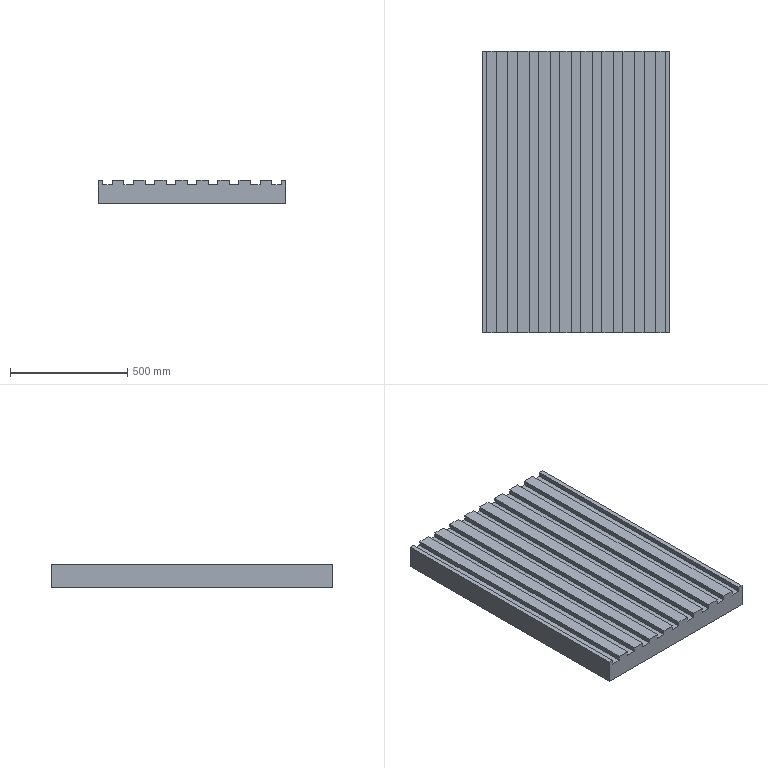Part | SolidWorks | features Extrusion 1, ICE 1, LPattern 1 | 1 solid | 42 faces | box 800 x 1200 x 100 mm | volume 87360000 mm3 | plane 42
STEP:
#1=CARTESIAN_POINT('',(200.,-600.,100.));
#2=VERTEX_POINT('',#1);
#3=CARTESIAN_POINT('',(200.,600.,100.));
#4=VERTEX_POINT('',#3);
#5=CARTESIAN_POINT('',(200.,0.,100.));
#6=DIRECTION('',(0.,1.,0.));
#7=VECTOR('',#6,1000.);
#8=LINE('',#5,#7);
#9=EDGE_CURVE('',#2,#4,#8,.T.);
#10=ORIENTED_EDGE('',*,*,#9,.F.);
#11=CARTESIAN_POINT('',(250.,-600.,100.));
#12=VERTEX_POINT('',#11);
#13=CARTESIAN_POINT('',(-400.,-600.,100.));
#14=DIRECTION('',(1.,0.,0.));
#15=VECTOR('',#14,1000.);
#16=LINE('',#13,#15);
#17=EDGE_CURVE('',#2,#12,#16,.T.);
#18=ORIENTED_EDGE('',*,*,#17,.T.);
#19=CARTESIAN_POINT('',(250.,600.,100.));
#20=VERTEX_POINT('',#19);
#21=CARTESIAN_POINT('',(250.,0.,100.));
#22=DIRECTION('',(0.,-1.,0.));
#23=VECTOR('',#22,1000.);
#24=LINE('',#21,#23);
#25=EDGE_CURVE('',#20,#12,#24,.T.);
#26=ORIENTED_EDGE('',*,*,#25,.F.);
#27=CARTESIAN_POINT('',(-400.,600.,100.));
#28=DIRECTION('',(-1.,0.,0.));
#29=VECTOR('',#28,1000.);
#30=LINE('',#27,#29);
#31=EDGE_CURVE('',#20,#4,#30,.T.);
#32=ORIENTED_EDGE('',*,*,#31,.T.);
#33=EDGE_LOOP('',(#10,#18,#26,#32));
#34=FACE_OUTER_BOUND('',#33,.T.);
#35=CARTESIAN_POINT('',(0.,0.,100.));
#36=DIRECTION('',(0.,0.,1.));
#37=DIRECTION('',(1.,0.,0.));
#38=AXIS2_PLACEMENT_3D('',#35,#36,#37);
#39=PLANE('',#38);
#40=ADVANCED_FACE('',(#34),#39,.T.);
#41=CARTESIAN_POINT('',(290.,-600.,100.));
#42=VERTEX_POINT('',#41);
#43=CARTESIAN_POINT('',(290.,600.,100.));
#44=VERTEX_POINT('',#43);
#45=CARTESIAN_POINT('',(290.,0.,100.));
#46=DIRECTION('',(0.,1.,0.));
#47=VECTOR('',#46,1000.);
#48=LINE('',#45,#47);
#49=EDGE_CURVE('',#42,#44,#48,.T.);
#50=ORIENTED_EDGE('',*,*,#49,.F.);
#51=CARTESIAN_POINT('',(340.,-600.,100.));
#52=VERTEX_POINT('',#51);
#53=CARTESIAN_POINT('',(-400.,-600.,100.));
#54=DIRECTION('',(1.,0.,0.));
#55=VECTOR('',#54,1000.);
#56=LINE('',#53,#55);
#57=EDGE_CURVE('',#42,#52,#56,.T.);
#58=ORIENTED_EDGE('',*,*,#57,.T.);
#59=CARTESIAN_POINT('',(340.,600.,100.));
#60=VERTEX_POINT('',#59);
#61=CARTESIAN_POINT('',(340.,0.,100.));
#62=DIRECTION('',(0.,-1.,0.));
#63=VECTOR('',#62,1000.);
#64=LINE('',#61,#63);
#65=EDGE_CURVE('',#60,#52,#64,.T.);
#66=ORIENTED_EDGE('',*,*,#65,.F.);
#67=CARTESIAN_POINT('',(-400.,600.,100.));
#68=DIRECTION('',(-1.,0.,0.));
#69=VECTOR('',#68,1000.);
#70=LINE('',#67,#69);
#71=EDGE_CURVE('',#60,#44,#70,.T.);
#72=ORIENTED_EDGE('',*,*,#71,.T.);
#73=EDGE_LOOP('',(#50,#58,#66,#72));
#74=FACE_OUTER_BOUND('',#73,.T.);
#75=CARTESIAN_POINT('',(0.,0.,100.));
#76=DIRECTION('',(0.,0.,1.));
#77=DIRECTION('',(1.,0.,0.));
#78=AXIS2_PLACEMENT_3D('',#75,#76,#77);
#79=PLANE('',#78);
#80=ADVANCED_FACE('',(#74),#79,.T.);
#81=CARTESIAN_POINT('',(160.,600.,100.));
#82=VERTEX_POINT('',#81);
#83=CARTESIAN_POINT('',(160.,-600.,100.));
#84=VERTEX_POINT('',#83);
#85=CARTESIAN_POINT('',(160.,0.,100.));
#86=DIRECTION('',(0.,-1.,0.));
#87=VECTOR('',#86,1000.);
#88=LINE('',#85,#87);
#89=EDGE_CURVE('',#82,#84,#88,.T.);
#90=ORIENTED_EDGE('',*,*,#89,.F.);
#91=CARTESIAN_POINT('',(110.,600.,100.));
#92=VERTEX_POINT('',#91);
#93=CARTESIAN_POINT('',(-400.,600.,100.));
#94=DIRECTION('',(-1.,0.,0.));
#95=VECTOR('',#94,1000.);
#96=LINE('',#93,#95);
#97=EDGE_CURVE('',#82,#92,#96,.T.);
#98=ORIENTED_EDGE('',*,*,#97,.T.);
#99=CARTESIAN_POINT('',(110.,-600.,100.));
#100=VERTEX_POINT('',#99);
#101=CARTESIAN_POINT('',(110.,0.,100.));
#102=DIRECTION('',(0.,1.,0.));
#103=VECTOR('',#102,1000.);
#104=LINE('',#101,#103);
#105=EDGE_CURVE('',#100,#92,#104,.T.);
#106=ORIENTED_EDGE('',*,*,#105,.F.);
#107=CARTESIAN_POINT('',(-400.,-600.,100.));
#108=DIRECTION('',(1.,0.,0.));
#109=VECTOR('',#108,1000.);
#110=LINE('',#107,#109);
#111=EDGE_CURVE('',#100,#84,#110,.T.);
#112=ORIENTED_EDGE('',*,*,#111,.T.);
#113=EDGE_LOOP('',(#90,#98,#106,#112));
#114=FACE_OUTER_BOUND('',#113,.T.);
#115=CARTESIAN_POINT('',(0.,0.,100.));
#116=DIRECTION('',(0.,0.,1.));
#117=DIRECTION('',(1.,0.,0.));
#118=AXIS2_PLACEMENT_3D('',#115,#116,#117);
#119=PLANE('',#118);
#120=ADVANCED_FACE('',(#114),#119,.T.);
#121=CARTESIAN_POINT('',(380.,-600.,100.));
#122=VERTEX_POINT('',#121);
#123=CARTESIAN_POINT('',(380.,600.,100.));
#124=VERTEX_POINT('',#123);
#125=CARTESIAN_POINT('',(380.,0.,100.));
#126=DIRECTION('',(0.,1.,0.));
#127=VECTOR('',#126,1000.);
#128=LINE('',#125,#127);
#129=EDGE_CURVE('',#122,#124,#128,.T.);
#130=ORIENTED_EDGE('',*,*,#129,.F.);
#131=CARTESIAN_POINT('',(400.,-600.,100.));
#132=VERTEX_POINT('',#131);
#133=CARTESIAN_POINT('',(-400.,-600.,100.));
#134=DIRECTION('',(1.,0.,0.));
#135=VECTOR('',#134,1000.);
#136=LINE('',#133,#135);
#137=EDGE_CURVE('',#122,#132,#136,.T.);
#138=ORIENTED_EDGE('',*,*,#137,.T.);
#139=CARTESIAN_POINT('',(400.,600.,100.));
#140=VERTEX_POINT('',#139);
#141=CARTESIAN_POINT('',(400.,600.,100.));
#142=DIRECTION('',(0.,1.,0.));
#143=VECTOR('',#142,1000.);
#144=LINE('',#141,#143);
#145=EDGE_CURVE('',#132,#140,#144,.T.);
#146=ORIENTED_EDGE('',*,*,#145,.T.);
#147=CARTESIAN_POINT('',(-400.,600.,100.));
#148=DIRECTION('',(-1.,0.,0.));
#149=VECTOR('',#148,1000.);
#150=LINE('',#147,#149);
#151=EDGE_CURVE('',#140,#124,#150,.T.);
#152=ORIENTED_EDGE('',*,*,#151,.T.);
#153=EDGE_LOOP('',(#130,#138,#146,#152));
#154=FACE_OUTER_BOUND('',#153,.T.);
#155=CARTESIAN_POINT('',(0.,0.,100.));
#156=DIRECTION('',(0.,0.,1.));
#157=DIRECTION('',(1.,0.,0.));
#158=AXIS2_PLACEMENT_3D('',#155,#156,#157);
#159=PLANE('',#158);
#160=ADVANCED_FACE('',(#154),#159,.T.);
#161=CARTESIAN_POINT('',(-340.,-600.,100.));
#162=VERTEX_POINT('',#161);
#163=CARTESIAN_POINT('',(-340.,600.,100.));
#164=VERTEX_POINT('',#163);
#165=CARTESIAN_POINT('',(-340.,0.,100.));
#166=DIRECTION('',(0.,1.,0.));
#167=VECTOR('',#166,1000.);
#168=LINE('',#165,#167);
#169=EDGE_CURVE('',#162,#164,#168,.T.);
#170=ORIENTED_EDGE('',*,*,#169,.F.);
#171=CARTESIAN_POINT('',(-290.,-600.,100.));
#172=VERTEX_POINT('',#171);
#173=CARTESIAN_POINT('',(-400.,-600.,100.));
#174=DIRECTION('',(1.,0.,0.));
#175=VECTOR('',#174,1000.);
#176=LINE('',#173,#175);
#177=EDGE_CURVE('',#162,#172,#176,.T.);
#178=ORIENTED_EDGE('',*,*,#177,.T.);
#179=CARTESIAN_POINT('',(-290.,600.,100.));
#180=VERTEX_POINT('',#179);
#181=CARTESIAN_POINT('',(-290.,0.,100.));
#182=DIRECTION('',(0.,-1.,0.));
#183=VECTOR('',#182,1000.);
#184=LINE('',#181,#183);
#185=EDGE_CURVE('',#180,#172,#184,.T.);
#186=ORIENTED_EDGE('',*,*,#185,.F.);
#187=CARTESIAN_POINT('',(-400.,600.,100.));
#188=DIRECTION('',(-1.,0.,0.));
#189=VECTOR('',#188,1000.);
#190=LINE('',#187,#189);
#191=EDGE_CURVE('',#180,#164,#190,.T.);
#192=ORIENTED_EDGE('',*,*,#191,.T.);
#193=EDGE_LOOP('',(#170,#178,#186,#192));
#194=FACE_OUTER_BOUND('',#193,.T.);
#195=CARTESIAN_POINT('',(0.,0.,100.));
#196=DIRECTION('',(0.,0.,1.));
#197=DIRECTION('',(1.,0.,0.));
#198=AXIS2_PLACEMENT_3D('',#195,#196,#197);
#199=PLANE('',#198);
#200=ADVANCED_FACE('',(#194),#199,.T.);
#201=CARTESIAN_POINT('',(-250.,-600.,100.));
#202=VERTEX_POINT('',#201);
#203=CARTESIAN_POINT('',(-250.,600.,100.));
#204=VERTEX_POINT('',#203);
#205=CARTESIAN_POINT('',(-250.,0.,100.));
#206=DIRECTION('',(0.,1.,0.));
#207=VECTOR('',#206,1000.);
#208=LINE('',#205,#207);
#209=EDGE_CURVE('',#202,#204,#208,.T.);
#210=ORIENTED_EDGE('',*,*,#209,.F.);
#211=CARTESIAN_POINT('',(-200.,-600.,100.));
#212=VERTEX_POINT('',#211);
#213=CARTESIAN_POINT('',(-400.,-600.,100.));
#214=DIRECTION('',(1.,0.,0.));
#215=VECTOR('',#214,1000.);
#216=LINE('',#213,#215);
#217=EDGE_CURVE('',#202,#212,#216,.T.);
#218=ORIENTED_EDGE('',*,*,#217,.T.);
#219=CARTESIAN_POINT('',(-200.,600.,100.));
#220=VERTEX_POINT('',#219);
#221=CARTESIAN_POINT('',(-200.,0.,100.));
#222=DIRECTION('',(0.,-1.,0.));
#223=VECTOR('',#222,1000.);
#224=LINE('',#221,#223);
#225=EDGE_CURVE('',#220,#212,#224,.T.);
#226=ORIENTED_EDGE('',*,*,#225,.F.);
#227=CARTESIAN_POINT('',(-400.,600.,100.));
#228=DIRECTION('',(-1.,0.,0.));
#229=VECTOR('',#228,1000.);
#230=LINE('',#227,#229);
#231=EDGE_CURVE('',#220,#204,#230,.T.);
#232=ORIENTED_EDGE('',*,*,#231,.T.);
#233=EDGE_LOOP('',(#210,#218,#226,#232));
#234=FACE_OUTER_BOUND('',#233,.T.);
#235=CARTESIAN_POINT('',(0.,0.,100.));
#236=DIRECTION('',(0.,0.,1.));
#237=DIRECTION('',(1.,0.,0.));
#238=AXIS2_PLACEMENT_3D('',#235,#236,#237);
#239=PLANE('',#238);
#240=ADVANCED_FACE('',(#234),#239,.T.);
#241=CARTESIAN_POINT('',(-160.,-600.,100.));
#242=VERTEX_POINT('',#241);
#243=CARTESIAN_POINT('',(-160.,600.,100.));
#244=VERTEX_POINT('',#243);
#245=CARTESIAN_POINT('',(-160.,0.,100.));
#246=DIRECTION('',(0.,1.,0.));
#247=VECTOR('',#246,1000.);
#248=LINE('',#245,#247);
#249=EDGE_CURVE('',#242,#244,#248,.T.);
#250=ORIENTED_EDGE('',*,*,#249,.F.);
#251=CARTESIAN_POINT('',(-110.,-600.,100.));
#252=VERTEX_POINT('',#251);
#253=CARTESIAN_POINT('',(-400.,-600.,100.));
#254=DIRECTION('',(1.,0.,0.));
#255=VECTOR('',#254,1000.);
#256=LINE('',#253,#255);
#257=EDGE_CURVE('',#242,#252,#256,.T.);
#258=ORIENTED_EDGE('',*,*,#257,.T.);
#259=CARTESIAN_POINT('',(-110.,600.,100.));
#260=VERTEX_POINT('',#259);
#261=CARTESIAN_POINT('',(-110.,0.,100.));
#262=DIRECTION('',(0.,-1.,0.));
#263=VECTOR('',#262,1000.);
#264=LINE('',#261,#263);
#265=EDGE_CURVE('',#260,#252,#264,.T.);
#266=ORIENTED_EDGE('',*,*,#265,.F.);
#267=CARTESIAN_POINT('',(-400.,600.,100.));
#268=DIRECTION('',(-1.,0.,0.));
#269=VECTOR('',#268,1000.);
#270=LINE('',#267,#269);
#271=EDGE_CURVE('',#260,#244,#270,.T.);
#272=ORIENTED_EDGE('',*,*,#271,.T.);
#273=EDGE_LOOP('',(#250,#258,#266,#272));
#274=FACE_OUTER_BOUND('',#273,.T.);
#275=CARTESIAN_POINT('',(0.,0.,100.));
#276=DIRECTION('',(0.,0.,1.));
#277=DIRECTION('',(1.,0.,0.));
#278=AXIS2_PLACEMENT_3D('',#275,#276,#277);
#279=PLANE('',#278);
#280=ADVANCED_FACE('',(#274),#279,.T.);
#281=CARTESIAN_POINT('',(-70.,-600.,100.));
#282=VERTEX_POINT('',#281);
#283=CARTESIAN_POINT('',(-70.,600.,100.));
#284=VERTEX_POINT('',#283);
#285=CARTESIAN_POINT('',(-70.,0.,100.));
#286=DIRECTION('',(0.,1.,0.));
#287=VECTOR('',#286,1000.);
#288=LINE('',#285,#287);
#289=EDGE_CURVE('',#282,#284,#288,.T.);
#290=ORIENTED_EDGE('',*,*,#289,.F.);
#291=CARTESIAN_POINT('',(-20.,-600.,100.));
#292=VERTEX_POINT('',#291);
#293=CARTESIAN_POINT('',(-400.,-600.,100.));
#294=DIRECTION('',(1.,0.,0.));
#295=VECTOR('',#294,1000.);
#296=LINE('',#293,#295);
#297=EDGE_CURVE('',#282,#292,#296,.T.);
#298=ORIENTED_EDGE('',*,*,#297,.T.);
#299=CARTESIAN_POINT('',(-20.,600.,100.));
#300=VERTEX_POINT('',#299);
#301=CARTESIAN_POINT('',(-20.,0.,100.));
#302=DIRECTION('',(0.,-1.,0.));
#303=VECTOR('',#302,1000.);
#304=LINE('',#301,#303);
#305=EDGE_CURVE('',#300,#292,#304,.T.);
#306=ORIENTED_EDGE('',*,*,#305,.F.);
#307=CARTESIAN_POINT('',(-400.,600.,100.));
#308=DIRECTION('',(-1.,0.,0.));
#309=VECTOR('',#308,1000.);
#310=LINE('',#307,#309);
#311=EDGE_CURVE('',#300,#284,#310,.T.);
#312=ORIENTED_EDGE('',*,*,#311,.T.);
#313=EDGE_LOOP('',(#290,#298,#306,#312));
#314=FACE_OUTER_BOUND('',#313,.T.);
#315=CARTESIAN_POINT('',(0.,0.,100.));
#316=DIRECTION('',(0.,0.,1.));
#317=DIRECTION('',(1.,0.,0.));
#318=AXIS2_PLACEMENT_3D('',#315,#316,#317);
#319=PLANE('',#318);
#320=ADVANCED_FACE('',(#314),#319,.T.);
#321=CARTESIAN_POINT('',(70.,600.,100.));
#322=VERTEX_POINT('',#321);
#323=CARTESIAN_POINT('',(70.,-600.,100.));
#324=VERTEX_POINT('',#323);
#325=CARTESIAN_POINT('',(70.,0.,100.));
#326=DIRECTION('',(0.,-1.,0.));
#327=VECTOR('',#326,1000.);
#328=LINE('',#325,#327);
#329=EDGE_CURVE('',#322,#324,#328,.T.);
#330=ORIENTED_EDGE('',*,*,#329,.F.);
#331=CARTESIAN_POINT('',(20.,600.,100.));
#332=VERTEX_POINT('',#331);
#333=CARTESIAN_POINT('',(-400.,600.,100.));
#334=DIRECTION('',(-1.,0.,0.));
#335=VECTOR('',#334,1000.);
#336=LINE('',#333,#335);
#337=EDGE_CURVE('',#322,#332,#336,.T.);
#338=ORIENTED_EDGE('',*,*,#337,.T.);
#339=CARTESIAN_POINT('',(20.,-600.,100.));
#340=VERTEX_POINT('',#339);
#341=CARTESIAN_POINT('',(20.,0.,100.));
#342=DIRECTION('',(0.,1.,0.));
#343=VECTOR('',#342,1000.);
#344=LINE('',#341,#343);
#345=EDGE_CURVE('',#340,#332,#344,.T.);
#346=ORIENTED_EDGE('',*,*,#345,.F.);
#347=CARTESIAN_POINT('',(-400.,-600.,100.));
#348=DIRECTION('',(1.,0.,0.));
#349=VECTOR('',#348,1000.);
#350=LINE('',#347,#349);
#351=EDGE_CURVE('',#340,#324,#350,.T.);
#352=ORIENTED_EDGE('',*,*,#351,.T.);
#353=EDGE_LOOP('',(#330,#338,#346,#352));
#354=FACE_OUTER_BOUND('',#353,.T.);
#355=CARTESIAN_POINT('',(0.,0.,100.));
#356=DIRECTION('',(0.,0.,1.));
#357=DIRECTION('',(1.,0.,0.));
#358=AXIS2_PLACEMENT_3D('',#355,#356,#357);
#359=PLANE('',#358);
#360=ADVANCED_FACE('',(#354),#359,.T.);
#361=CARTESIAN_POINT('',(400.,-600.,0.));
#362=VERTEX_POINT('',#361);
#363=CARTESIAN_POINT('',(400.,600.,0.));
#364=VERTEX_POINT('',#363);
#365=CARTESIAN_POINT('',(400.,600.,0.));
#366=DIRECTION('',(0.,1.,0.));
#367=VECTOR('',#366,1000.);
#368=LINE('',#365,#367);
#369=EDGE_CURVE('',#362,#364,#368,.T.);
#370=ORIENTED_EDGE('',*,*,#369,.T.);
#371=CARTESIAN_POINT('',(400.,600.,100.));
#372=DIRECTION('',(0.,0.,-1.));
#373=VECTOR('',#372,1000.);
#374=LINE('',#371,#373);
#375=EDGE_CURVE('',#140,#364,#374,.T.);
#376=ORIENTED_EDGE('',*,*,#375,.F.);
#377=ORIENTED_EDGE('',*,*,#145,.F.);
#378=CARTESIAN_POINT('',(400.,-600.,100.));
#379=DIRECTION('',(0.,0.,-1.));
#380=VECTOR('',#379,1000.);
#381=LINE('',#378,#380);
#382=EDGE_CURVE('',#132,#362,#381,.T.);
#383=ORIENTED_EDGE('',*,*,#382,.T.);
#384=EDGE_LOOP('',(#370,#376,#377,#383));
#385=FACE_OUTER_BOUND('',#384,.T.);
#386=CARTESIAN_POINT('',(400.,600.,100.));
#387=DIRECTION('',(-1.,0.,0.));
#388=DIRECTION('',(0.,-1.,0.));
#389=AXIS2_PLACEMENT_3D('',#386,#387,#388);
#390=PLANE('',#389);
#391=ADVANCED_FACE('',(#385),#390,.F.);
#392=CARTESIAN_POINT('',(160.,600.,80.));
#393=VERTEX_POINT('',#392);
#394=CARTESIAN_POINT('',(200.,600.,80.));
#395=VERTEX_POINT('',#394);
#396=CARTESIAN_POINT('',(160.,600.,80.));
#397=DIRECTION('',(1.,0.,0.));
#398=VECTOR('',#397,1000.);
#399=LINE('',#396,#398);
#400=EDGE_CURVE('',#393,#395,#399,.T.);
#401=ORIENTED_EDGE('',*,*,#400,.T.);
#402=CARTESIAN_POINT('',(200.,600.,120.));
#403=DIRECTION('',(0.,0.,1.));
#404=VECTOR('',#403,1000.);
#405=LINE('',#402,#404);
#406=EDGE_CURVE('',#395,#4,#405,.T.);
#407=ORIENTED_EDGE('',*,*,#406,.T.);
#408=ORIENTED_EDGE('',*,*,#31,.F.);
#409=CARTESIAN_POINT('',(250.,600.,80.));
#410=VERTEX_POINT('',#409);
#411=CARTESIAN_POINT('',(250.,600.,120.));
#412=DIRECTION('',(0.,0.,-1.));
#413=VECTOR('',#412,1000.);
#414=LINE('',#411,#413);
#415=EDGE_CURVE('',#20,#410,#414,.T.);
#416=ORIENTED_EDGE('',*,*,#415,.T.);
#417=CARTESIAN_POINT('',(290.,600.,80.));
#418=VERTEX_POINT('',#417);
#419=CARTESIAN_POINT('',(250.,600.,80.));
#420=DIRECTION('',(1.,0.,0.));
#421=VECTOR('',#420,1000.);
#422=LINE('',#419,#421);
#423=EDGE_CURVE('',#410,#418,#422,.T.);
#424=ORIENTED_EDGE('',*,*,#423,.T.);
#425=CARTESIAN_POINT('',(290.,600.,120.));
#426=DIRECTION('',(0.,0.,1.));
#427=VECTOR('',#426,1000.);
#428=LINE('',#425,#427);
#429=EDGE_CURVE('',#418,#44,#428,.T.);
#430=ORIENTED_EDGE('',*,*,#429,.T.);
#431=ORIENTED_EDGE('',*,*,#71,.F.);
#432=CARTESIAN_POINT('',(340.,600.,80.));
#433=VERTEX_POINT('',#432);
#434=CARTESIAN_POINT('',(340.,600.,120.));
#435=DIRECTION('',(0.,0.,-1.));
#436=VECTOR('',#435,1000.);
#437=LINE('',#434,#436);
#438=EDGE_CURVE('',#60,#433,#437,.T.);
#439=ORIENTED_EDGE('',*,*,#438,.T.);
#440=CARTESIAN_POINT('',(380.,600.,80.));
#441=VERTEX_POINT('',#440);
#442=CARTESIAN_POINT('',(340.,600.,80.));
#443=DIRECTION('',(1.,0.,0.));
#444=VECTOR('',#443,1000.);
#445=LINE('',#442,#444);
#446=EDGE_CURVE('',#433,#441,#445,.T.);
#447=ORIENTED_EDGE('',*,*,#446,.T.);
#448=CARTESIAN_POINT('',(380.,600.,120.));
#449=DIRECTION('',(0.,0.,1.));
#450=VECTOR('',#449,1000.);
#451=LINE('',#448,#450);
#452=EDGE_CURVE('',#441,#124,#451,.T.);
#453=ORIENTED_EDGE('',*,*,#452,.T.);
#454=ORIENTED_EDGE('',*,*,#151,.F.);
#455=ORIENTED_EDGE('',*,*,#375,.T.);
#456=CARTESIAN_POINT('',(-400.,600.,0.));
#457=VERTEX_POINT('',#456);
#458=CARTESIAN_POINT('',(-400.,600.,0.));
#459=DIRECTION('',(-1.,0.,0.));
#460=VECTOR('',#459,1000.);
#461=LINE('',#458,#460);
#462=EDGE_CURVE('',#364,#457,#461,.T.);
#463=ORIENTED_EDGE('',*,*,#462,.T.);
#464=CARTESIAN_POINT('',(-400.,600.,100.));
#465=VERTEX_POINT('',#464);
#466=CARTESIAN_POINT('',(-400.,600.,100.));
#467=DIRECTION('',(0.,0.,-1.));
#468=VECTOR('',#467,1000.);
#469=LINE('',#466,#468);
#470=EDGE_CURVE('',#465,#457,#469,.T.);
#471=ORIENTED_EDGE('',*,*,#470,.F.);
#472=CARTESIAN_POINT('',(-380.,600.,100.));
#473=VERTEX_POINT('',#472);
#474=CARTESIAN_POINT('',(-400.,600.,100.));
#475=DIRECTION('',(-1.,0.,0.));
#476=VECTOR('',#475,1000.);
#477=LINE('',#474,#476);
#478=EDGE_CURVE('',#473,#465,#477,.T.);
#479=ORIENTED_EDGE('',*,*,#478,.F.);
#480=CARTESIAN_POINT('',(-380.,600.,80.));
#481=VERTEX_POINT('',#480);
#482=CARTESIAN_POINT('',(-380.,600.,120.));
#483=DIRECTION('',(0.,0.,-1.));
#484=VECTOR('',#483,1000.);
#485=LINE('',#482,#484);
#486=EDGE_CURVE('',#473,#481,#485,.T.);
#487=ORIENTED_EDGE('',*,*,#486,.T.);
#488=CARTESIAN_POINT('',(-340.,600.,80.));
#489=VERTEX_POINT('',#488);
#490=CARTESIAN_POINT('',(-380.,600.,80.));
#491=DIRECTION('',(1.,0.,0.));
#492=VECTOR('',#491,1000.);
#493=LINE('',#490,#492);
#494=EDGE_CURVE('',#481,#489,#493,.T.);
#495=ORIENTED_EDGE('',*,*,#494,.T.);
#496=CARTESIAN_POINT('',(-340.,600.,120.));
#497=DIRECTION('',(0.,0.,1.));
#498=VECTOR('',#497,1000.);
#499=LINE('',#496,#498);
#500=EDGE_CURVE('',#489,#164,#499,.T.);
#501=ORIENTED_EDGE('',*,*,#500,.T.);
#502=ORIENTED_EDGE('',*,*,#191,.F.);
#503=CARTESIAN_POINT('',(-290.,600.,80.));
#504=VERTEX_POINT('',#503);
#505=CARTESIAN_POINT('',(-290.,600.,120.));
#506=DIRECTION('',(0.,0.,-1.));
#507=VECTOR('',#506,1000.);
#508=LINE('',#505,#507);
#509=EDGE_CURVE('',#180,#504,#508,.T.);
#510=ORIENTED_EDGE('',*,*,#509,.T.);
#511=CARTESIAN_POINT('',(-250.,600.,80.));
#512=VERTEX_POINT('',#511);
#513=CARTESIAN_POINT('',(-290.,600.,80.));
#514=DIRECTION('',(1.,0.,0.));
#515=VECTOR('',#514,1000.);
#516=LINE('',#513,#515);
#517=EDGE_CURVE('',#504,#512,#516,.T.);
#518=ORIENTED_EDGE('',*,*,#517,.T.);
#519=CARTESIAN_POINT('',(-250.,600.,120.));
#520=DIRECTION('',(0.,0.,1.));
#521=VECTOR('',#520,1000.);
#522=LINE('',#519,#521);
#523=EDGE_CURVE('',#512,#204,#522,.T.);
#524=ORIENTED_EDGE('',*,*,#523,.T.);
#525=ORIENTED_EDGE('',*,*,#231,.F.);
#526=CARTESIAN_POINT('',(-200.,600.,80.));
#527=VERTEX_POINT('',#526);
#528=CARTESIAN_POINT('',(-200.,600.,120.));
#529=DIRECTION('',(0.,0.,-1.));
#530=VECTOR('',#529,1000.);
#531=LINE('',#528,#530);
#532=EDGE_CURVE('',#220,#527,#531,.T.);
#533=ORIENTED_EDGE('',*,*,#532,.T.);
#534=CARTESIAN_POINT('',(-160.,600.,80.));
#535=VERTEX_POINT('',#534);
#536=CARTESIAN_POINT('',(-200.,600.,80.));
#537=DIRECTION('',(1.,0.,0.));
#538=VECTOR('',#537,1000.);
#539=LINE('',#536,#538);
#540=EDGE_CURVE('',#527,#535,#539,.T.);
#541=ORIENTED_EDGE('',*,*,#540,.T.);
#542=CARTESIAN_POINT('',(-160.,600.,120.));
#543=DIRECTION('',(0.,0.,1.));
#544=VECTOR('',#543,1000.);
#545=LINE('',#542,#544);
#546=EDGE_CURVE('',#535,#244,#545,.T.);
#547=ORIENTED_EDGE('',*,*,#546,.T.);
#548=ORIENTED_EDGE('',*,*,#271,.F.);
#549=CARTESIAN_POINT('',(-110.,600.,80.));
#550=VERTEX_POINT('',#549);
#551=CARTESIAN_POINT('',(-110.,600.,120.));
#552=DIRECTION('',(0.,0.,-1.));
#553=VECTOR('',#552,1000.);
#554=LINE('',#551,#553);
#555=EDGE_CURVE('',#260,#550,#554,.T.);
#556=ORIENTED_EDGE('',*,*,#555,.T.);
#557=CARTESIAN_POINT('',(-70.,600.,80.));
#558=VERTEX_POINT('',#557);
#559=CARTESIAN_POINT('',(-110.,600.,80.));
#560=DIRECTION('',(1.,0.,0.));
#561=VECTOR('',#560,1000.);
#562=LINE('',#559,#561);
#563=EDGE_CURVE('',#550,#558,#562,.T.);
#564=ORIENTED_EDGE('',*,*,#563,.T.);
#565=CARTESIAN_POINT('',(-70.,600.,120.));
#566=DIRECTION('',(0.,0.,1.));
#567=VECTOR('',#566,1000.);
#568=LINE('',#565,#567);
#569=EDGE_CURVE('',#558,#284,#568,.T.);
#570=ORIENTED_EDGE('',*,*,#569,.T.);
#571=ORIENTED_EDGE('',*,*,#311,.F.);
#572=CARTESIAN_POINT('',(-20.,600.,80.));
#573=VERTEX_POINT('',#572);
#574=CARTESIAN_POINT('',(-20.,600.,120.));
#575=DIRECTION('',(0.,0.,-1.));
#576=VECTOR('',#575,1000.);
#577=LINE('',#574,#576);
#578=EDGE_CURVE('',#300,#573,#577,.T.);
#579=ORIENTED_EDGE('',*,*,#578,.T.);
#580=CARTESIAN_POINT('',(20.,600.,80.));
#581=VERTEX_POINT('',#580);
#582=CARTESIAN_POINT('',(-20.,600.,80.));
#583=DIRECTION('',(1.,0.,0.));
#584=VECTOR('',#583,1000.);
#585=LINE('',#582,#584);
#586=EDGE_CURVE('',#573,#581,#585,.T.);
#587=ORIENTED_EDGE('',*,*,#586,.T.);
#588=CARTESIAN_POINT('',(20.,600.,120.));
#589=DIRECTION('',(0.,0.,1.));
#590=VECTOR('',#589,1000.);
#591=LINE('',#588,#590);
#592=EDGE_CURVE('',#581,#332,#591,.T.);
#593=ORIENTED_EDGE('',*,*,#592,.T.);
#594=ORIENTED_EDGE('',*,*,#337,.F.);
#595=CARTESIAN_POINT('',(70.,600.,80.));
#596=VERTEX_POINT('',#595);
#597=CARTESIAN_POINT('',(70.,600.,120.));
#598=DIRECTION('',(0.,0.,-1.));
#599=VECTOR('',#598,1000.);
#600=LINE('',#597,#599);
#601=EDGE_CURVE('',#322,#596,#600,.T.);
#602=ORIENTED_EDGE('',*,*,#601,.T.);
#603=CARTESIAN_POINT('',(110.,600.,80.));
#604=VERTEX_POINT('',#603);
#605=CARTESIAN_POINT('',(70.,600.,80.));
#606=DIRECTION('',(1.,0.,0.));
#607=VECTOR('',#606,1000.);
#608=LINE('',#605,#607);
#609=EDGE_CURVE('',#596,#604,#608,.T.);
#610=ORIENTED_EDGE('',*,*,#609,.T.);
#611=CARTESIAN_POINT('',(110.,600.,120.));
#612=DIRECTION('',(0.,0.,1.));
#613=VECTOR('',#612,1000.);
#614=LINE('',#611,#613);
#615=EDGE_CURVE('',#604,#92,#614,.T.);
#616=ORIENTED_EDGE('',*,*,#615,.T.);
#617=ORIENTED_EDGE('',*,*,#97,.F.);
#618=CARTESIAN_POINT('',(160.,600.,120.));
#619=DIRECTION('',(0.,0.,-1.));
#620=VECTOR('',#619,1000.);
#621=LINE('',#618,#620);
#622=EDGE_CURVE('',#82,#393,#621,.T.);
#623=ORIENTED_EDGE('',*,*,#622,.T.);
#624=EDGE_LOOP('',(#401,#407,#408,#416,#424,#430,#431,#439,#447,#453,#454,#455,#463,#471,#479,#487,#495,#501,#502,#510,#518,#524,#525,#533,#541,#547,#548,#556,#564,#570,#571,#579,#587,#593,#594,#602,#610,#616,#617,#623));
#625=FACE_OUTER_BOUND('',#624,.T.);
#626=CARTESIAN_POINT('',(-400.,600.,100.));
#627=DIRECTION('',(0.,-1.,0.));
#628=DIRECTION('',(0.,0.,-1.));
#629=AXIS2_PLACEMENT_3D('',#626,#627,#628);
#630=PLANE('',#629);
#631=ADVANCED_FACE('',(#625),#630,.F.);
#632=CARTESIAN_POINT('',(-400.,-600.,0.));
#633=VERTEX_POINT('',#632);
#634=CARTESIAN_POINT('',(-400.,600.,0.));
#635=DIRECTION('',(0.,-1.,0.));
#636=VECTOR('',#635,1000.);
#637=LINE('',#634,#636);
#638=EDGE_CURVE('',#457,#633,#637,.T.);
#639=ORIENTED_EDGE('',*,*,#638,.T.);
#640=CARTESIAN_POINT('',(-400.,-600.,100.));
#641=VERTEX_POINT('',#640);
#642=CARTESIAN_POINT('',(-400.,-600.,100.));
#643=DIRECTION('',(0.,0.,-1.));
#644=VECTOR('',#643,1000.);
#645=LINE('',#642,#644);
#646=EDGE_CURVE('',#641,#633,#645,.T.);
#647=ORIENTED_EDGE('',*,*,#646,.F.);
#648=CARTESIAN_POINT('',(-400.,600.,100.));
#649=DIRECTION('',(0.,-1.,0.));
#650=VECTOR('',#649,1000.);
#651=LINE('',#648,#650);
#652=EDGE_CURVE('',#465,#641,#651,.T.);
#653=ORIENTED_EDGE('',*,*,#652,.F.);
#654=ORIENTED_EDGE('',*,*,#470,.T.);
#655=EDGE_LOOP('',(#639,#647,#653,#654));
#656=FACE_OUTER_BOUND('',#655,.T.);
#657=CARTESIAN_POINT('',(-400.,600.,100.));
#658=DIRECTION('',(1.,0.,0.));
#659=DIRECTION('',(0.,1.,0.));
#660=AXIS2_PLACEMENT_3D('',#657,#658,#659);
#661=PLANE('',#660);
#662=ADVANCED_FACE('',(#656),#661,.F.);
#663=ORIENTED_EDGE('',*,*,#17,.F.);
#664=CARTESIAN_POINT('',(200.,-600.,80.));
#665=VERTEX_POINT('',#664);
#666=CARTESIAN_POINT('',(200.,-600.,120.));
#667=DIRECTION('',(0.,0.,1.));
#668=VECTOR('',#667,1000.);
#669=LINE('',#666,#668);
#670=EDGE_CURVE('',#665,#2,#669,.T.);
#671=ORIENTED_EDGE('',*,*,#670,.F.);
#672=CARTESIAN_POINT('',(160.,-600.,80.));
#673=VERTEX_POINT('',#672);
#674=CARTESIAN_POINT('',(160.,-600.,80.));
#675=DIRECTION('',(1.,0.,0.));
#676=VECTOR('',#675,1000.);
#677=LINE('',#674,#676);
#678=EDGE_CURVE('',#673,#665,#677,.T.);
#679=ORIENTED_EDGE('',*,*,#678,.F.);
#680=CARTESIAN_POINT('',(160.,-600.,100.));
#681=DIRECTION('',(0.,0.,1.));
#682=VECTOR('',#681,1000.);
#683=LINE('',#680,#682);
#684=EDGE_CURVE('',#673,#84,#683,.T.);
#685=ORIENTED_EDGE('',*,*,#684,.T.);
#686=ORIENTED_EDGE('',*,*,#111,.F.);
#687=CARTESIAN_POINT('',(110.,-600.,80.));
#688=VERTEX_POINT('',#687);
#689=CARTESIAN_POINT('',(110.,-600.,120.));
#690=DIRECTION('',(0.,0.,1.));
#691=VECTOR('',#690,1000.);
#692=LINE('',#689,#691);
#693=EDGE_CURVE('',#688,#100,#692,.T.);
#694=ORIENTED_EDGE('',*,*,#693,.F.);
#695=CARTESIAN_POINT('',(70.,-600.,80.));
#696=VERTEX_POINT('',#695);
#697=CARTESIAN_POINT('',(70.,-600.,80.));
#698=DIRECTION('',(1.,0.,0.));
#699=VECTOR('',#698,1000.);
#700=LINE('',#697,#699);
#701=EDGE_CURVE('',#696,#688,#700,.T.);
#702=ORIENTED_EDGE('',*,*,#701,.F.);
#703=CARTESIAN_POINT('',(70.,-600.,100.));
#704=DIRECTION('',(0.,0.,1.));
#705=VECTOR('',#704,1000.);
#706=LINE('',#703,#705);
#707=EDGE_CURVE('',#696,#324,#706,.T.);
#708=ORIENTED_EDGE('',*,*,#707,.T.);
#709=ORIENTED_EDGE('',*,*,#351,.F.);
#710=CARTESIAN_POINT('',(20.,-600.,80.));
#711=VERTEX_POINT('',#710);
#712=CARTESIAN_POINT('',(20.,-600.,120.));
#713=DIRECTION('',(0.,0.,1.));
#714=VECTOR('',#713,1000.);
#715=LINE('',#712,#714);
#716=EDGE_CURVE('',#711,#340,#715,.T.);
#717=ORIENTED_EDGE('',*,*,#716,.F.);
#718=CARTESIAN_POINT('',(-20.,-600.,80.));
#719=VERTEX_POINT('',#718);
#720=CARTESIAN_POINT('',(-20.,-600.,80.));
#721=DIRECTION('',(1.,0.,0.));
#722=VECTOR('',#721,1000.);
#723=LINE('',#720,#722);
#724=EDGE_CURVE('',#719,#711,#723,.T.);
#725=ORIENTED_EDGE('',*,*,#724,.F.);
#726=CARTESIAN_POINT('',(-20.,-600.,120.));
#727=DIRECTION('',(0.,0.,-1.));
#728=VECTOR('',#727,1000.);
#729=LINE('',#726,#728);
#730=EDGE_CURVE('',#292,#719,#729,.T.);
#731=ORIENTED_EDGE('',*,*,#730,.F.);
#732=ORIENTED_EDGE('',*,*,#297,.F.);
#733=CARTESIAN_POINT('',(-70.,-600.,80.));
#734=VERTEX_POINT('',#733);
#735=CARTESIAN_POINT('',(-70.,-600.,120.));
#736=DIRECTION('',(0.,0.,1.));
#737=VECTOR('',#736,1000.);
#738=LINE('',#735,#737);
#739=EDGE_CURVE('',#734,#282,#738,.T.);
#740=ORIENTED_EDGE('',*,*,#739,.F.);
#741=CARTESIAN_POINT('',(-110.,-600.,80.));
#742=VERTEX_POINT('',#741);
#743=CARTESIAN_POINT('',(-110.,-600.,80.));
#744=DIRECTION('',(1.,0.,0.));
#745=VECTOR('',#744,1000.);
#746=LINE('',#743,#745);
#747=EDGE_CURVE('',#742,#734,#746,.T.);
#748=ORIENTED_EDGE('',*,*,#747,.F.);
#749=CARTESIAN_POINT('',(-110.,-600.,120.));
#750=DIRECTION('',(0.,0.,-1.));
#751=VECTOR('',#750,1000.);
#752=LINE('',#749,#751);
#753=EDGE_CURVE('',#252,#742,#752,.T.);
#754=ORIENTED_EDGE('',*,*,#753,.F.);
#755=ORIENTED_EDGE('',*,*,#257,.F.);
#756=CARTESIAN_POINT('',(-160.,-600.,80.));
#757=VERTEX_POINT('',#756);
#758=CARTESIAN_POINT('',(-160.,-600.,120.));
#759=DIRECTION('',(0.,0.,1.));
#760=VECTOR('',#759,1000.);
#761=LINE('',#758,#760);
#762=EDGE_CURVE('',#757,#242,#761,.T.);
#763=ORIENTED_EDGE('',*,*,#762,.F.);
#764=CARTESIAN_POINT('',(-200.,-600.,80.));
#765=VERTEX_POINT('',#764);
#766=CARTESIAN_POINT('',(-200.,-600.,80.));
#767=DIRECTION('',(1.,0.,0.));
#768=VECTOR('',#767,1000.);
#769=LINE('',#766,#768);
#770=EDGE_CURVE('',#765,#757,#769,.T.);
#771=ORIENTED_EDGE('',*,*,#770,.F.);
#772=CARTESIAN_POINT('',(-200.,-600.,120.));
#773=DIRECTION('',(0.,0.,-1.));
#774=VECTOR('',#773,1000.);
#775=LINE('',#772,#774);
#776=EDGE_CURVE('',#212,#765,#775,.T.);
#777=ORIENTED_EDGE('',*,*,#776,.F.);
#778=ORIENTED_EDGE('',*,*,#217,.F.);
#779=CARTESIAN_POINT('',(-250.,-600.,80.));
#780=VERTEX_POINT('',#779);
#781=CARTESIAN_POINT('',(-250.,-600.,120.));
#782=DIRECTION('',(0.,0.,1.));
#783=VECTOR('',#782,1000.);
#784=LINE('',#781,#783);
#785=EDGE_CURVE('',#780,#202,#784,.T.);
#786=ORIENTED_EDGE('',*,*,#785,.F.);
#787=CARTESIAN_POINT('',(-290.,-600.,80.));
#788=VERTEX_POINT('',#787);
#789=CARTESIAN_POINT('',(-290.,-600.,80.));
#790=DIRECTION('',(1.,0.,0.));
#791=VECTOR('',#790,1000.);
#792=LINE('',#789,#791);
#793=EDGE_CURVE('',#788,#780,#792,.T.);
#794=ORIENTED_EDGE('',*,*,#793,.F.);
#795=CARTESIAN_POINT('',(-290.,-600.,120.));
#796=DIRECTION('',(0.,0.,-1.));
#797=VECTOR('',#796,1000.);
#798=LINE('',#795,#797);
#799=EDGE_CURVE('',#172,#788,#798,.T.);
#800=ORIENTED_EDGE('',*,*,#799,.F.);
#801=ORIENTED_EDGE('',*,*,#177,.F.);
#802=CARTESIAN_POINT('',(-340.,-600.,80.));
#803=VERTEX_POINT('',#802);
#804=CARTESIAN_POINT('',(-340.,-600.,120.));
#805=DIRECTION('',(0.,0.,1.));
#806=VECTOR('',#805,1000.);
#807=LINE('',#804,#806);
#808=EDGE_CURVE('',#803,#162,#807,.T.);
#809=ORIENTED_EDGE('',*,*,#808,.F.);
#810=CARTESIAN_POINT('',(-380.,-600.,80.));
#811=VERTEX_POINT('',#810);
#812=CARTESIAN_POINT('',(-380.,-600.,80.));
#813=DIRECTION('',(1.,0.,0.));
#814=VECTOR('',#813,1000.);
#815=LINE('',#812,#814);
#816=EDGE_CURVE('',#811,#803,#815,.T.);
#817=ORIENTED_EDGE('',*,*,#816,.F.);
#818=CARTESIAN_POINT('',(-380.,-600.,100.));
#819=VERTEX_POINT('',#818);
#820=CARTESIAN_POINT('',(-380.,-600.,120.));
#821=DIRECTION('',(0.,0.,-1.));
#822=VECTOR('',#821,1000.);
#823=LINE('',#820,#822);
#824=EDGE_CURVE('',#819,#811,#823,.T.);
#825=ORIENTED_EDGE('',*,*,#824,.F.);
#826=CARTESIAN_POINT('',(-400.,-600.,100.));
#827=DIRECTION('',(1.,0.,0.));
#828=VECTOR('',#827,1000.);
#829=LINE('',#826,#828);
#830=EDGE_CURVE('',#641,#819,#829,.T.);
#831=ORIENTED_EDGE('',*,*,#830,.F.);
#832=ORIENTED_EDGE('',*,*,#646,.T.);
#833=CARTESIAN_POINT('',(-400.,-600.,0.));
#834=DIRECTION('',(1.,0.,0.));
#835=VECTOR('',#834,1000.);
#836=LINE('',#833,#835);
#837=EDGE_CURVE('',#633,#362,#836,.T.);
#838=ORIENTED_EDGE('',*,*,#837,.T.);
#839=ORIENTED_EDGE('',*,*,#382,.F.);
#840=ORIENTED_EDGE('',*,*,#137,.F.);
#841=CARTESIAN_POINT('',(380.,-600.,80.));
#842=VERTEX_POINT('',#841);
#843=CARTESIAN_POINT('',(380.,-600.,120.));
#844=DIRECTION('',(0.,0.,1.));
#845=VECTOR('',#844,1000.);
#846=LINE('',#843,#845);
#847=EDGE_CURVE('',#842,#122,#846,.T.);
#848=ORIENTED_EDGE('',*,*,#847,.F.);
#849=CARTESIAN_POINT('',(340.,-600.,80.));
#850=VERTEX_POINT('',#849);
#851=CARTESIAN_POINT('',(340.,-600.,80.));
#852=DIRECTION('',(1.,0.,0.));
#853=VECTOR('',#852,1000.);
#854=LINE('',#851,#853);
#855=EDGE_CURVE('',#850,#842,#854,.T.);
#856=ORIENTED_EDGE('',*,*,#855,.F.);
#857=CARTESIAN_POINT('',(340.,-600.,100.));
#858=DIRECTION('',(0.,0.,1.));
#859=VECTOR('',#858,1000.);
#860=LINE('',#857,#859);
#861=EDGE_CURVE('',#850,#52,#860,.T.);
#862=ORIENTED_EDGE('',*,*,#861,.T.);
#863=ORIENTED_EDGE('',*,*,#57,.F.);
#864=CARTESIAN_POINT('',(290.,-600.,80.));
#865=VERTEX_POINT('',#864);
#866=CARTESIAN_POINT('',(290.,-600.,120.));
#867=DIRECTION('',(0.,0.,1.));
#868=VECTOR('',#867,1000.);
#869=LINE('',#866,#868);
#870=EDGE_CURVE('',#865,#42,#869,.T.);
#871=ORIENTED_EDGE('',*,*,#870,.F.);
#872=CARTESIAN_POINT('',(250.,-600.,80.));
#873=VERTEX_POINT('',#872);
#874=CARTESIAN_POINT('',(250.,-600.,80.));
#875=DIRECTION('',(1.,0.,0.));
#876=VECTOR('',#875,1000.);
#877=LINE('',#874,#876);
#878=EDGE_CURVE('',#873,#865,#877,.T.);
#879=ORIENTED_EDGE('',*,*,#878,.F.);
#880=CARTESIAN_POINT('',(250.,-600.,100.));
#881=DIRECTION('',(0.,0.,1.));
#882=VECTOR('',#881,1000.);
#883=LINE('',#880,#882);
#884=EDGE_CURVE('',#873,#12,#883,.T.);
#885=ORIENTED_EDGE('',*,*,#884,.T.);
#886=EDGE_LOOP('',(#663,#671,#679,#685,#686,#694,#702,#708,#709,#717,#725,#731,#732,#740,#748,#754,#755,#763,#771,#777,#778,#786,#794,#800,#801,#809,#817,#825,#831,#832,#838,#839,#840,#848,#856,#862,#863,#871,#879,#885));
#887=FACE_OUTER_BOUND('',#886,.T.);
#888=CARTESIAN_POINT('',(-400.,-600.,100.));
#889=DIRECTION('',(0.,1.,0.));
#890=DIRECTION('',(0.,0.,1.));
#891=AXIS2_PLACEMENT_3D('',#888,#889,#890);
#892=PLANE('',#891);
#893=ADVANCED_FACE('',(#887),#892,.F.);
#894=CARTESIAN_POINT('',(-380.,0.,100.));
#895=DIRECTION('',(0.,-1.,0.));
#896=VECTOR('',#895,1000.);
#897=LINE('',#894,#896);
#898=EDGE_CURVE('',#473,#819,#897,.T.);
#899=ORIENTED_EDGE('',*,*,#898,.F.);
#900=ORIENTED_EDGE('',*,*,#478,.T.);
#901=ORIENTED_EDGE('',*,*,#652,.T.);
#902=ORIENTED_EDGE('',*,*,#830,.T.);
#903=EDGE_LOOP('',(#899,#900,#901,#902));
#904=FACE_OUTER_BOUND('',#903,.T.);
#905=CARTESIAN_POINT('',(0.,0.,100.));
#906=DIRECTION('',(0.,0.,1.));
#907=DIRECTION('',(1.,0.,0.));
#908=AXIS2_PLACEMENT_3D('',#905,#906,#907);
#909=PLANE('',#908);
#910=ADVANCED_FACE('',(#904),#909,.T.);
#911=ORIENTED_EDGE('',*,*,#369,.F.);
#912=ORIENTED_EDGE('',*,*,#837,.F.);
#913=ORIENTED_EDGE('',*,*,#638,.F.);
#914=ORIENTED_EDGE('',*,*,#462,.F.);
#915=EDGE_LOOP('',(#911,#912,#913,#914));
#916=FACE_OUTER_BOUND('',#915,.T.);
#917=CARTESIAN_POINT('',(0.,0.,0.));
#918=DIRECTION('',(0.,0.,1.));
#919=DIRECTION('',(1.,0.,0.));
#920=AXIS2_PLACEMENT_3D('',#917,#918,#919);
#921=PLANE('',#920);
#922=ADVANCED_FACE('',(#916),#921,.F.);
#923=ORIENTED_EDGE('',*,*,#345,.T.);
#924=ORIENTED_EDGE('',*,*,#592,.F.);
#925=CARTESIAN_POINT('',(20.,600.,80.));
#926=DIRECTION('',(0.,-1.,0.));
#927=VECTOR('',#926,1000.);
#928=LINE('',#925,#927);
#929=EDGE_CURVE('',#581,#711,#928,.T.);
#930=ORIENTED_EDGE('',*,*,#929,.T.);
#931=ORIENTED_EDGE('',*,*,#716,.T.);
#932=EDGE_LOOP('',(#923,#924,#930,#931));
#933=FACE_OUTER_BOUND('',#932,.T.);
#934=CARTESIAN_POINT('',(20.,600.,120.));
#935=DIRECTION('',(1.,0.,0.));
#936=DIRECTION('',(0.,0.,-1.));
#937=AXIS2_PLACEMENT_3D('',#934,#935,#936);
#938=PLANE('',#937);
#939=ADVANCED_FACE('',(#933),#938,.F.);
#940=ORIENTED_EDGE('',*,*,#724,.T.);
#941=ORIENTED_EDGE('',*,*,#929,.F.);
#942=ORIENTED_EDGE('',*,*,#586,.F.);
#943=CARTESIAN_POINT('',(-20.,600.,80.));
#944=DIRECTION('',(0.,-1.,0.));
#945=VECTOR('',#944,1000.);
#946=LINE('',#943,#945);
#947=EDGE_CURVE('',#573,#719,#946,.T.);
#948=ORIENTED_EDGE('',*,*,#947,.T.);
#949=EDGE_LOOP('',(#940,#941,#942,#948));
#950=FACE_OUTER_BOUND('',#949,.T.);
#951=CARTESIAN_POINT('',(-20.,600.,80.));
#952=DIRECTION('',(0.,0.,-1.));
#953=DIRECTION('',(-1.,0.,0.));
#954=AXIS2_PLACEMENT_3D('',#951,#952,#953);
#955=PLANE('',#954);
#956=ADVANCED_FACE('',(#950),#955,.F.);
#957=ORIENTED_EDGE('',*,*,#305,.T.);
#958=ORIENTED_EDGE('',*,*,#730,.T.);
#959=ORIENTED_EDGE('',*,*,#947,.F.);
#960=ORIENTED_EDGE('',*,*,#578,.F.);
#961=EDGE_LOOP('',(#957,#958,#959,#960));
#962=FACE_OUTER_BOUND('',#961,.T.);
#963=CARTESIAN_POINT('',(-20.,600.,120.));
#964=DIRECTION('',(-1.,0.,0.));
#965=DIRECTION('',(0.,0.,1.));
#966=AXIS2_PLACEMENT_3D('',#963,#964,#965);
#967=PLANE('',#966);
#968=ADVANCED_FACE('',(#962),#967,.F.);
#969=ORIENTED_EDGE('',*,*,#289,.T.);
#970=ORIENTED_EDGE('',*,*,#569,.F.);
#971=CARTESIAN_POINT('',(-70.,600.,80.));
#972=DIRECTION('',(0.,-1.,0.));
#973=VECTOR('',#972,1000.);
#974=LINE('',#971,#973);
#975=EDGE_CURVE('',#558,#734,#974,.T.);
#976=ORIENTED_EDGE('',*,*,#975,.T.);
#977=ORIENTED_EDGE('',*,*,#739,.T.);
#978=EDGE_LOOP('',(#969,#970,#976,#977));
#979=FACE_OUTER_BOUND('',#978,.T.);
#980=CARTESIAN_POINT('',(-70.,600.,120.));
#981=DIRECTION('',(1.,0.,0.));
#982=DIRECTION('',(0.,0.,-1.));
#983=AXIS2_PLACEMENT_3D('',#980,#981,#982);
#984=PLANE('',#983);
#985=ADVANCED_FACE('',(#979),#984,.F.);
#986=ORIENTED_EDGE('',*,*,#747,.T.);
#987=ORIENTED_EDGE('',*,*,#975,.F.);
#988=ORIENTED_EDGE('',*,*,#563,.F.);
#989=CARTESIAN_POINT('',(-110.,600.,80.));
#990=DIRECTION('',(0.,-1.,0.));
#991=VECTOR('',#990,1000.);
#992=LINE('',#989,#991);
#993=EDGE_CURVE('',#550,#742,#992,.T.);
#994=ORIENTED_EDGE('',*,*,#993,.T.);
#995=EDGE_LOOP('',(#986,#987,#988,#994));
#996=FACE_OUTER_BOUND('',#995,.T.);
#997=CARTESIAN_POINT('',(-110.,600.,80.));
#998=DIRECTION('',(0.,0.,-1.));
#999=DIRECTION('',(-1.,0.,0.));
#1000=AXIS2_PLACEMENT_3D('',#997,#998,#999);
#1001=PLANE('',#1000);
#1002=ADVANCED_FACE('',(#996),#1001,.F.);
#1003=ORIENTED_EDGE('',*,*,#265,.T.);
#1004=ORIENTED_EDGE('',*,*,#753,.T.);
#1005=ORIENTED_EDGE('',*,*,#993,.F.);
#1006=ORIENTED_EDGE('',*,*,#555,.F.);
#1007=EDGE_LOOP('',(#1003,#1004,#1005,#1006));
#1008=FACE_OUTER_BOUND('',#1007,.T.);
#1009=CARTESIAN_POINT('',(-110.,600.,120.));
#1010=DIRECTION('',(-1.,0.,0.));
#1011=DIRECTION('',(0.,0.,1.));
#1012=AXIS2_PLACEMENT_3D('',#1009,#1010,#1011);
#1013=PLANE('',#1012);
#1014=ADVANCED_FACE('',(#1008),#1013,.F.);
#1015=ORIENTED_EDGE('',*,*,#249,.T.);
#1016=ORIENTED_EDGE('',*,*,#546,.F.);
#1017=CARTESIAN_POINT('',(-160.,600.,80.));
#1018=DIRECTION('',(0.,-1.,0.));
#1019=VECTOR('',#1018,1000.);
#1020=LINE('',#1017,#1019);
#1021=EDGE_CURVE('',#535,#757,#1020,.T.);
#1022=ORIENTED_EDGE('',*,*,#1021,.T.);
#1023=ORIENTED_EDGE('',*,*,#762,.T.);
#1024=EDGE_LOOP('',(#1015,#1016,#1022,#1023));
#1025=FACE_OUTER_BOUND('',#1024,.T.);
#1026=CARTESIAN_POINT('',(-160.,600.,120.));
#1027=DIRECTION('',(1.,0.,0.));
#1028=DIRECTION('',(0.,0.,-1.));
#1029=AXIS2_PLACEMENT_3D('',#1026,#1027,#1028);
#1030=PLANE('',#1029);
#1031=ADVANCED_FACE('',(#1025),#1030,.F.);
#1032=ORIENTED_EDGE('',*,*,#770,.T.);
#1033=ORIENTED_EDGE('',*,*,#1021,.F.);
#1034=ORIENTED_EDGE('',*,*,#540,.F.);
#1035=CARTESIAN_POINT('',(-200.,600.,80.));
#1036=DIRECTION('',(0.,-1.,0.));
#1037=VECTOR('',#1036,1000.);
#1038=LINE('',#1035,#1037);
#1039=EDGE_CURVE('',#527,#765,#1038,.T.);
#1040=ORIENTED_EDGE('',*,*,#1039,.T.);
#1041=EDGE_LOOP('',(#1032,#1033,#1034,#1040));
#1042=FACE_OUTER_BOUND('',#1041,.T.);
#1043=CARTESIAN_POINT('',(-200.,600.,80.));
#1044=DIRECTION('',(0.,0.,-1.));
#1045=DIRECTION('',(-1.,0.,0.));
#1046=AXIS2_PLACEMENT_3D('',#1043,#1044,#1045);
#1047=PLANE('',#1046);
#1048=ADVANCED_FACE('',(#1042),#1047,.F.);
#1049=ORIENTED_EDGE('',*,*,#225,.T.);
#1050=ORIENTED_EDGE('',*,*,#776,.T.);
#1051=ORIENTED_EDGE('',*,*,#1039,.F.);
#1052=ORIENTED_EDGE('',*,*,#532,.F.);
#1053=EDGE_LOOP('',(#1049,#1050,#1051,#1052));
#1054=FACE_OUTER_BOUND('',#1053,.T.);
#1055=CARTESIAN_POINT('',(-200.,600.,120.));
#1056=DIRECTION('',(-1.,0.,0.));
#1057=DIRECTION('',(0.,0.,1.));
#1058=AXIS2_PLACEMENT_3D('',#1055,#1056,#1057);
#1059=PLANE('',#1058);
#1060=ADVANCED_FACE('',(#1054),#1059,.F.);
#1061=ORIENTED_EDGE('',*,*,#209,.T.);
#1062=ORIENTED_EDGE('',*,*,#523,.F.);
#1063=CARTESIAN_POINT('',(-250.,600.,80.));
#1064=DIRECTION('',(0.,-1.,0.));
#1065=VECTOR('',#1064,1000.);
#1066=LINE('',#1063,#1065);
#1067=EDGE_CURVE('',#512,#780,#1066,.T.);
#1068=ORIENTED_EDGE('',*,*,#1067,.T.);
#1069=ORIENTED_EDGE('',*,*,#785,.T.);
#1070=EDGE_LOOP('',(#1061,#1062,#1068,#1069));
#1071=FACE_OUTER_BOUND('',#1070,.T.);
#1072=CARTESIAN_POINT('',(-250.,600.,120.));
#1073=DIRECTION('',(1.,0.,0.));
#1074=DIRECTION('',(0.,0.,-1.));
#1075=AXIS2_PLACEMENT_3D('',#1072,#1073,#1074);
#1076=PLANE('',#1075);
#1077=ADVANCED_FACE('',(#1071),#1076,.F.);
#1078=ORIENTED_EDGE('',*,*,#793,.T.);
#1079=ORIENTED_EDGE('',*,*,#1067,.F.);
#1080=ORIENTED_EDGE('',*,*,#517,.F.);
#1081=CARTESIAN_POINT('',(-290.,600.,80.));
#1082=DIRECTION('',(0.,-1.,0.));
#1083=VECTOR('',#1082,1000.);
#1084=LINE('',#1081,#1083);
#1085=EDGE_CURVE('',#504,#788,#1084,.T.);
#1086=ORIENTED_EDGE('',*,*,#1085,.T.);
#1087=EDGE_LOOP('',(#1078,#1079,#1080,#1086));
#1088=FACE_OUTER_BOUND('',#1087,.T.);
#1089=CARTESIAN_POINT('',(-290.,600.,80.));
#1090=DIRECTION('',(0.,0.,-1.));
#1091=DIRECTION('',(-1.,0.,0.));
#1092=AXIS2_PLACEMENT_3D('',#1089,#1090,#1091);
#1093=PLANE('',#1092);
#1094=ADVANCED_FACE('',(#1088),#1093,.F.);
#1095=ORIENTED_EDGE('',*,*,#185,.T.);
#1096=ORIENTED_EDGE('',*,*,#799,.T.);
#1097=ORIENTED_EDGE('',*,*,#1085,.F.);
#1098=ORIENTED_EDGE('',*,*,#509,.F.);
#1099=EDGE_LOOP('',(#1095,#1096,#1097,#1098));
#1100=FACE_OUTER_BOUND('',#1099,.T.);
#1101=CARTESIAN_POINT('',(-290.,600.,120.));
#1102=DIRECTION('',(-1.,0.,0.));
#1103=DIRECTION('',(0.,0.,1.));
#1104=AXIS2_PLACEMENT_3D('',#1101,#1102,#1103);
#1105=PLANE('',#1104);
#1106=ADVANCED_FACE('',(#1100),#1105,.F.);
#1107=ORIENTED_EDGE('',*,*,#169,.T.);
#1108=ORIENTED_EDGE('',*,*,#500,.F.);
#1109=CARTESIAN_POINT('',(-340.,600.,80.));
#1110=DIRECTION('',(0.,-1.,0.));
#1111=VECTOR('',#1110,1000.);
#1112=LINE('',#1109,#1111);
#1113=EDGE_CURVE('',#489,#803,#1112,.T.);
#1114=ORIENTED_EDGE('',*,*,#1113,.T.);
#1115=ORIENTED_EDGE('',*,*,#808,.T.);
#1116=EDGE_LOOP('',(#1107,#1108,#1114,#1115));
#1117=FACE_OUTER_BOUND('',#1116,.T.);
#1118=CARTESIAN_POINT('',(-340.,600.,120.));
#1119=DIRECTION('',(1.,0.,0.));
#1120=DIRECTION('',(0.,0.,-1.));
#1121=AXIS2_PLACEMENT_3D('',#1118,#1119,#1120);
#1122=PLANE('',#1121);
#1123=ADVANCED_FACE('',(#1117),#1122,.F.);
#1124=ORIENTED_EDGE('',*,*,#816,.T.);
#1125=ORIENTED_EDGE('',*,*,#1113,.F.);
#1126=ORIENTED_EDGE('',*,*,#494,.F.);
#1127=CARTESIAN_POINT('',(-380.,600.,80.));
#1128=DIRECTION('',(0.,-1.,0.));
#1129=VECTOR('',#1128,1000.);
#1130=LINE('',#1127,#1129);
#1131=EDGE_CURVE('',#481,#811,#1130,.T.);
#1132=ORIENTED_EDGE('',*,*,#1131,.T.);
#1133=EDGE_LOOP('',(#1124,#1125,#1126,#1132));
#1134=FACE_OUTER_BOUND('',#1133,.T.);
#1135=CARTESIAN_POINT('',(-380.,600.,80.));
#1136=DIRECTION('',(0.,0.,-1.));
#1137=DIRECTION('',(-1.,0.,0.));
#1138=AXIS2_PLACEMENT_3D('',#1135,#1136,#1137);
#1139=PLANE('',#1138);
#1140=ADVANCED_FACE('',(#1134),#1139,.F.);
#1141=ORIENTED_EDGE('',*,*,#898,.T.);
#1142=ORIENTED_EDGE('',*,*,#824,.T.);
#1143=ORIENTED_EDGE('',*,*,#1131,.F.);
#1144=ORIENTED_EDGE('',*,*,#486,.F.);
#1145=EDGE_LOOP('',(#1141,#1142,#1143,#1144));
#1146=FACE_OUTER_BOUND('',#1145,.T.);
#1147=CARTESIAN_POINT('',(-380.,600.,120.));
#1148=DIRECTION('',(-1.,0.,0.));
#1149=DIRECTION('',(0.,0.,1.));
#1150=AXIS2_PLACEMENT_3D('',#1147,#1148,#1149);
#1151=PLANE('',#1150);
#1152=ADVANCED_FACE('',(#1146),#1151,.F.);
#1153=ORIENTED_EDGE('',*,*,#129,.T.);
#1154=ORIENTED_EDGE('',*,*,#452,.F.);
#1155=CARTESIAN_POINT('',(380.,600.,80.));
#1156=DIRECTION('',(0.,-1.,0.));
#1157=VECTOR('',#1156,1000.);
#1158=LINE('',#1155,#1157);
#1159=EDGE_CURVE('',#441,#842,#1158,.T.);
#1160=ORIENTED_EDGE('',*,*,#1159,.T.);
#1161=ORIENTED_EDGE('',*,*,#847,.T.);
#1162=EDGE_LOOP('',(#1153,#1154,#1160,#1161));
#1163=FACE_OUTER_BOUND('',#1162,.T.);
#1164=CARTESIAN_POINT('',(380.,600.,120.));
#1165=DIRECTION('',(1.,0.,0.));
#1166=DIRECTION('',(0.,0.,-1.));
#1167=AXIS2_PLACEMENT_3D('',#1164,#1165,#1166);
#1168=PLANE('',#1167);
#1169=ADVANCED_FACE('',(#1163),#1168,.F.);
#1170=ORIENTED_EDGE('',*,*,#855,.T.);
#1171=ORIENTED_EDGE('',*,*,#1159,.F.);
#1172=ORIENTED_EDGE('',*,*,#446,.F.);
#1173=CARTESIAN_POINT('',(340.,600.,80.));
#1174=DIRECTION('',(0.,-1.,0.));
#1175=VECTOR('',#1174,1000.);
#1176=LINE('',#1173,#1175);
#1177=EDGE_CURVE('',#433,#850,#1176,.T.);
#1178=ORIENTED_EDGE('',*,*,#1177,.T.);
#1179=EDGE_LOOP('',(#1170,#1171,#1172,#1178));
#1180=FACE_OUTER_BOUND('',#1179,.T.);
#1181=CARTESIAN_POINT('',(340.,600.,80.));
#1182=DIRECTION('',(0.,0.,-1.));
#1183=DIRECTION('',(-1.,0.,0.));
#1184=AXIS2_PLACEMENT_3D('',#1181,#1182,#1183);
#1185=PLANE('',#1184);
#1186=ADVANCED_FACE('',(#1180),#1185,.F.);
#1187=ORIENTED_EDGE('',*,*,#65,.T.);
#1188=ORIENTED_EDGE('',*,*,#861,.F.);
#1189=ORIENTED_EDGE('',*,*,#1177,.F.);
#1190=ORIENTED_EDGE('',*,*,#438,.F.);
#1191=EDGE_LOOP('',(#1187,#1188,#1189,#1190));
#1192=FACE_OUTER_BOUND('',#1191,.T.);
#1193=CARTESIAN_POINT('',(340.,600.,120.));
#1194=DIRECTION('',(-1.,0.,0.));
#1195=DIRECTION('',(0.,0.,1.));
#1196=AXIS2_PLACEMENT_3D('',#1193,#1194,#1195);
#1197=PLANE('',#1196);
#1198=ADVANCED_FACE('',(#1192),#1197,.F.);
#1199=ORIENTED_EDGE('',*,*,#105,.T.);
#1200=ORIENTED_EDGE('',*,*,#615,.F.);
#1201=CARTESIAN_POINT('',(110.,600.,80.));
#1202=DIRECTION('',(0.,-1.,0.));
#1203=VECTOR('',#1202,1000.);
#1204=LINE('',#1201,#1203);
#1205=EDGE_CURVE('',#604,#688,#1204,.T.);
#1206=ORIENTED_EDGE('',*,*,#1205,.T.);
#1207=ORIENTED_EDGE('',*,*,#693,.T.);
#1208=EDGE_LOOP('',(#1199,#1200,#1206,#1207));
#1209=FACE_OUTER_BOUND('',#1208,.T.);
#1210=CARTESIAN_POINT('',(110.,600.,120.));
#1211=DIRECTION('',(1.,0.,0.));
#1212=DIRECTION('',(0.,0.,-1.));
#1213=AXIS2_PLACEMENT_3D('',#1210,#1211,#1212);
#1214=PLANE('',#1213);
#1215=ADVANCED_FACE('',(#1209),#1214,.F.);
#1216=ORIENTED_EDGE('',*,*,#701,.T.);
#1217=ORIENTED_EDGE('',*,*,#1205,.F.);
#1218=ORIENTED_EDGE('',*,*,#609,.F.);
#1219=CARTESIAN_POINT('',(70.,600.,80.));
#1220=DIRECTION('',(0.,-1.,0.));
#1221=VECTOR('',#1220,1000.);
#1222=LINE('',#1219,#1221);
#1223=EDGE_CURVE('',#596,#696,#1222,.T.);
#1224=ORIENTED_EDGE('',*,*,#1223,.T.);
#1225=EDGE_LOOP('',(#1216,#1217,#1218,#1224));
#1226=FACE_OUTER_BOUND('',#1225,.T.);
#1227=CARTESIAN_POINT('',(70.,600.,80.));
#1228=DIRECTION('',(0.,0.,-1.));
#1229=DIRECTION('',(-1.,0.,0.));
#1230=AXIS2_PLACEMENT_3D('',#1227,#1228,#1229);
#1231=PLANE('',#1230);
#1232=ADVANCED_FACE('',(#1226),#1231,.F.);
#1233=ORIENTED_EDGE('',*,*,#329,.T.);
#1234=ORIENTED_EDGE('',*,*,#707,.F.);
#1235=ORIENTED_EDGE('',*,*,#1223,.F.);
#1236=ORIENTED_EDGE('',*,*,#601,.F.);
#1237=EDGE_LOOP('',(#1233,#1234,#1235,#1236));
#1238=FACE_OUTER_BOUND('',#1237,.T.);
#1239=CARTESIAN_POINT('',(70.,600.,120.));
#1240=DIRECTION('',(-1.,0.,0.));
#1241=DIRECTION('',(0.,0.,1.));
#1242=AXIS2_PLACEMENT_3D('',#1239,#1240,#1241);
#1243=PLANE('',#1242);
#1244=ADVANCED_FACE('',(#1238),#1243,.F.);
#1245=ORIENTED_EDGE('',*,*,#49,.T.);
#1246=ORIENTED_EDGE('',*,*,#429,.F.);
#1247=CARTESIAN_POINT('',(290.,600.,80.));
#1248=DIRECTION('',(0.,-1.,0.));
#1249=VECTOR('',#1248,1000.);
#1250=LINE('',#1247,#1249);
#1251=EDGE_CURVE('',#418,#865,#1250,.T.);
#1252=ORIENTED_EDGE('',*,*,#1251,.T.);
#1253=ORIENTED_EDGE('',*,*,#870,.T.);
#1254=EDGE_LOOP('',(#1245,#1246,#1252,#1253));
#1255=FACE_OUTER_BOUND('',#1254,.T.);
#1256=CARTESIAN_POINT('',(290.,600.,120.));
#1257=DIRECTION('',(1.,0.,0.));
#1258=DIRECTION('',(0.,0.,-1.));
#1259=AXIS2_PLACEMENT_3D('',#1256,#1257,#1258);
#1260=PLANE('',#1259);
#1261=ADVANCED_FACE('',(#1255),#1260,.F.);
#1262=ORIENTED_EDGE('',*,*,#878,.T.);
#1263=ORIENTED_EDGE('',*,*,#1251,.F.);
#1264=ORIENTED_EDGE('',*,*,#423,.F.);
#1265=CARTESIAN_POINT('',(250.,600.,80.));
#1266=DIRECTION('',(0.,-1.,0.));
#1267=VECTOR('',#1266,1000.);
#1268=LINE('',#1265,#1267);
#1269=EDGE_CURVE('',#410,#873,#1268,.T.);
#1270=ORIENTED_EDGE('',*,*,#1269,.T.);
#1271=EDGE_LOOP('',(#1262,#1263,#1264,#1270));
#1272=FACE_OUTER_BOUND('',#1271,.T.);
#1273=CARTESIAN_POINT('',(250.,600.,80.));
#1274=DIRECTION('',(0.,0.,-1.));
#1275=DIRECTION('',(-1.,0.,0.));
#1276=AXIS2_PLACEMENT_3D('',#1273,#1274,#1275);
#1277=PLANE('',#1276);
#1278=ADVANCED_FACE('',(#1272),#1277,.F.);
#1279=ORIENTED_EDGE('',*,*,#25,.T.);
#1280=ORIENTED_EDGE('',*,*,#884,.F.);
#1281=ORIENTED_EDGE('',*,*,#1269,.F.);
#1282=ORIENTED_EDGE('',*,*,#415,.F.);
#1283=EDGE_LOOP('',(#1279,#1280,#1281,#1282));
#1284=FACE_OUTER_BOUND('',#1283,.T.);
#1285=CARTESIAN_POINT('',(250.,600.,120.));
#1286=DIRECTION('',(-1.,0.,0.));
#1287=DIRECTION('',(0.,0.,1.));
#1288=AXIS2_PLACEMENT_3D('',#1285,#1286,#1287);
#1289=PLANE('',#1288);
#1290=ADVANCED_FACE('',(#1284),#1289,.F.);
#1291=ORIENTED_EDGE('',*,*,#9,.T.);
#1292=ORIENTED_EDGE('',*,*,#406,.F.);
#1293=CARTESIAN_POINT('',(200.,600.,80.));
#1294=DIRECTION('',(0.,-1.,0.));
#1295=VECTOR('',#1294,1000.);
#1296=LINE('',#1293,#1295);
#1297=EDGE_CURVE('',#395,#665,#1296,.T.);
#1298=ORIENTED_EDGE('',*,*,#1297,.T.);
#1299=ORIENTED_EDGE('',*,*,#670,.T.);
#1300=EDGE_LOOP('',(#1291,#1292,#1298,#1299));
#1301=FACE_OUTER_BOUND('',#1300,.T.);
#1302=CARTESIAN_POINT('',(200.,600.,120.));
#1303=DIRECTION('',(1.,0.,0.));
#1304=DIRECTION('',(0.,0.,-1.));
#1305=AXIS2_PLACEMENT_3D('',#1302,#1303,#1304);
#1306=PLANE('',#1305);
#1307=ADVANCED_FACE('',(#1301),#1306,.F.);
#1308=ORIENTED_EDGE('',*,*,#678,.T.);
#1309=ORIENTED_EDGE('',*,*,#1297,.F.);
#1310=ORIENTED_EDGE('',*,*,#400,.F.);
#1311=CARTESIAN_POINT('',(160.,600.,80.));
#1312=DIRECTION('',(0.,-1.,0.));
#1313=VECTOR('',#1312,1000.);
#1314=LINE('',#1311,#1313);
#1315=EDGE_CURVE('',#393,#673,#1314,.T.);
#1316=ORIENTED_EDGE('',*,*,#1315,.T.);
#1317=EDGE_LOOP('',(#1308,#1309,#1310,#1316));
#1318=FACE_OUTER_BOUND('',#1317,.T.);
#1319=CARTESIAN_POINT('',(160.,600.,80.));
#1320=DIRECTION('',(0.,0.,-1.));
#1321=DIRECTION('',(-1.,0.,0.));
#1322=AXIS2_PLACEMENT_3D('',#1319,#1320,#1321);
#1323=PLANE('',#1322);
#1324=ADVANCED_FACE('',(#1318),#1323,.F.);
#1325=ORIENTED_EDGE('',*,*,#89,.T.);
#1326=ORIENTED_EDGE('',*,*,#684,.F.);
#1327=ORIENTED_EDGE('',*,*,#1315,.F.);
#1328=ORIENTED_EDGE('',*,*,#622,.F.);
#1329=EDGE_LOOP('',(#1325,#1326,#1327,#1328));
#1330=FACE_OUTER_BOUND('',#1329,.T.);
#1331=CARTESIAN_POINT('',(160.,600.,120.));
#1332=DIRECTION('',(-1.,0.,0.));
#1333=DIRECTION('',(0.,0.,1.));
#1334=AXIS2_PLACEMENT_3D('',#1331,#1332,#1333);
#1335=PLANE('',#1334);
#1336=ADVANCED_FACE('',(#1330),#1335,.F.);
#1337=CLOSED_SHELL('',(#40,#80,#120,#160,#200,#240,#280,#320,#360,#391,#631,#662,#893,#910,#922,#939,#956,#968,#985,#1002,#1014,#1031,#1048,#1060,#1077,#1094,#1106,#1123,#1140,#1152,#1169,#1186,#1198,#1215,#1232,#1244,#1261,#1278,#1290,#1307,#1324,#1336));
#1338=MANIFOLD_SOLID_BREP('',#1337);
#1339=CARTESIAN_POINT('',(0.,0.,0.));
#1340=DIRECTION('',(0.,0.,1.));
#1341=DIRECTION('',(1.,0.,0.));
#1342=AXIS2_PLACEMENT_3D('',#1339,#1340,#1341);
#1343=(LENGTH_UNIT()NAMED_UNIT(*)SI_UNIT(.MILLI.,.METRE.));
#1344=UNCERTAINTY_MEASURE_WITH_UNIT(LENGTH_MEASURE(0.00001),#1343,'','');
#1345=(NAMED_UNIT(*)PLANE_ANGLE_UNIT()SI_UNIT($,.RADIAN.));
#1346=(NAMED_UNIT(*)SI_UNIT($,.STERADIAN.)SOLID_ANGLE_UNIT());
#1347=(GEOMETRIC_REPRESENTATION_CONTEXT(3)GLOBAL_UNCERTAINTY_ASSIGNED_CONTEXT((#1344))GLOBAL_UNIT_ASSIGNED_CONTEXT((#1343,#1345,#1346))REPRESENTATION_CONTEXT('',''));
#1348=ADVANCED_BREP_SHAPE_REPRESENTATION('',(#1338,#1342),#1347);